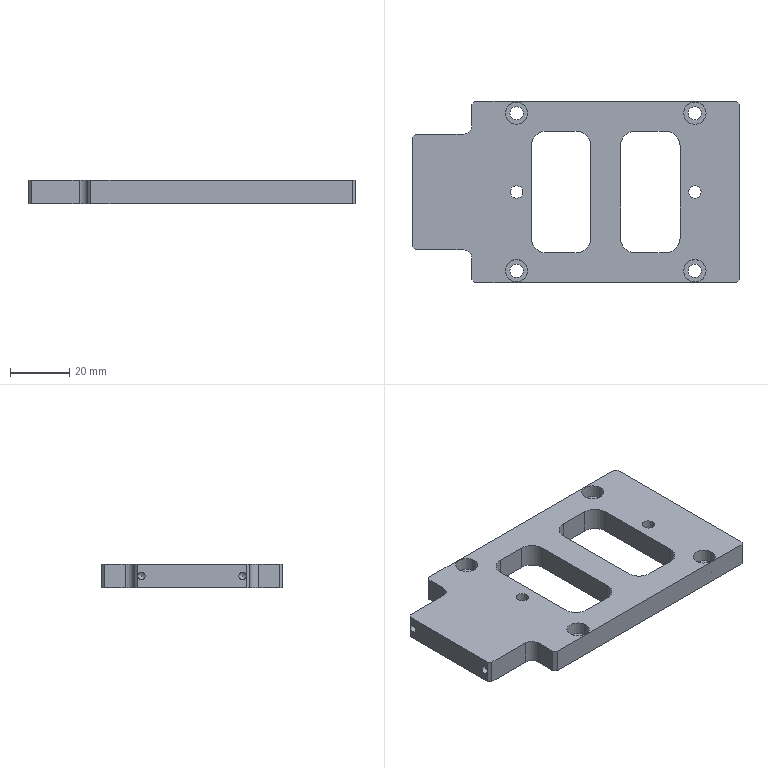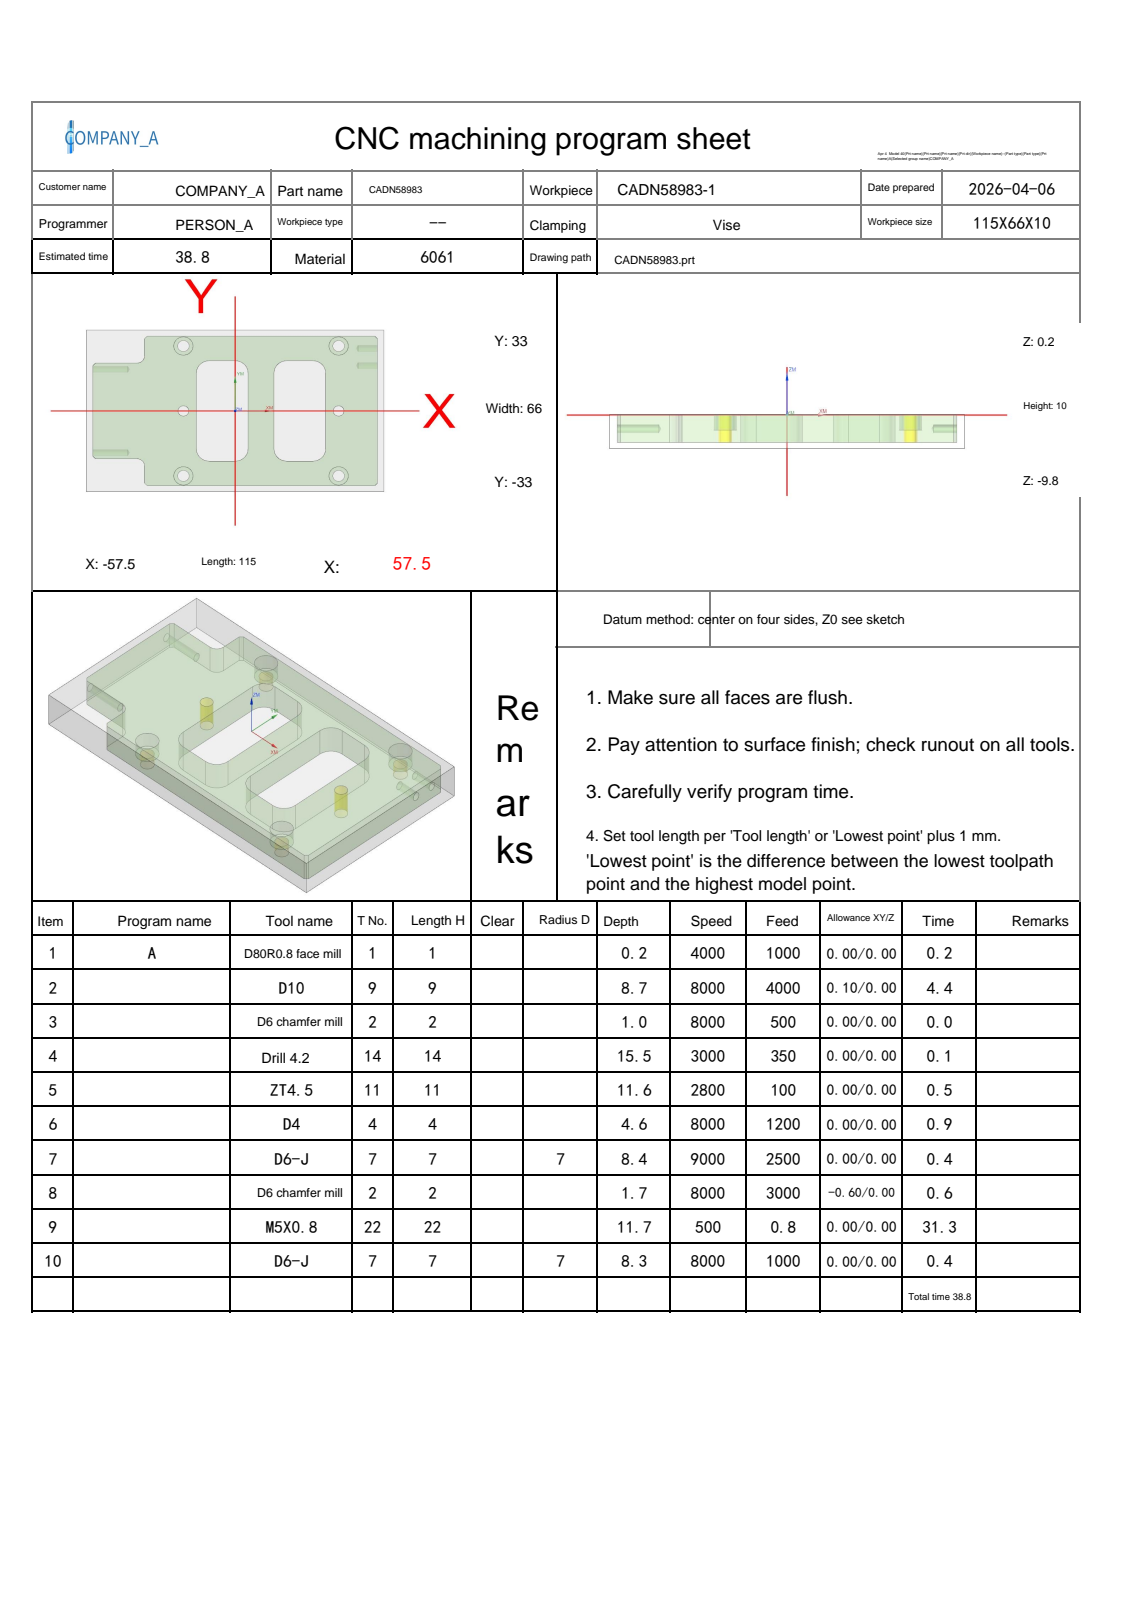NC program | NX | posted by the shop | part box 110 x 61 x 8 mm
Lines 35 to 2240 of 4510, first 1627 of 2206 lines:
N2 T09 M06
(D10  D=10. R=0. H=09 ce=0.10 di=0.10)
G00 G90 G54 X-39.25 Y-45. M03 S8000
G43 H09 Z10.2
M08
Z.724
G01 Z-.476 F4000.
Y-40.5
G03 X-46.25 Y-33.5 I-7. J0.0
G01 X-57.5
G02 X-58. Y-33. I0.0 J.5
G01 Y-24.623
G02 X-58.573 Y-24.119 I4. J5.123
X-59.617 Y-23.075 I9.382 J10.426
X-60.964 Y-21.085 I4.617 J4.575
X-61.5 Y-18.531 I5.813 J2.553
G01 Y-18.5
Y18.5
G02 X-61.492 Y18.823 I6.5 J0.0
X-60.858 Y21.317 I6.306 J-.276
X-59.618 Y23.075 I5.858 J-2.817
X-58.532 Y24.159 I10.618 J-9.54
X-58. Y24.623 I4.532 J-4.659
G01 Y33.
G02 X-57.5 Y33.5 I.5 J0.0
G01 X-41.699
G02 X-40.699 Y32.5 I0.0 J-1.
G01 X-40.713 Y32.333
X-41.614 Y27.005
X-41.627 Y26.838
G03 X-41.521 Y26.39 I1. J0.0
G01 X-41.5 Y26.301
Y26.199
G02 X-41.699 Y26. I-.2 J.001
G01 X-50.801
G02 X-51. Y26.199 I.001 J.2
G01 Y26.301
G02 X-50.801 Y26.5 I.2 J-.001
G01 X-44.983
G03 X-44.012 Y27.262 I0.0 J1.
G01 X-42.67 Y32.738
G02 X-41.699 Y33.5 I.971 J-.238
G01 X-40.123
G02 X-39.616 Y34.077 I5.123 J-4.
X-38.581 Y35.111 I11.116 J-10.081
X-36.645 Y36.438 I4.581 J-4.611
X-34.026 Y37. I2.619 J-5.815
G01 X54.
G02 X58.631 Y35.062 I0.0 J-6.5
G01 X59.596 Y34.096
G02 X61.482 Y29.977 I-4.596 J-4.596
X61.5 Y29.496 I-6.49 J-.482
G01 Y29.432
Y-29.5
G02 X59.596 Y-34.096 I-6.5 J0.0
G01 X58.596 Y-35.096
G02 X54. Y-37. I-4.596 J4.596
G01 X-34.
G02 X-38.596 Y-35.096 I0.0 J6.5
G01 X-39.596 Y-34.096
G02 X-40.123 Y-33.5 I4.596 J4.596
G01 X-51.25
G02 X-52.25 Y-32.5 I0.0 J1.
G01 X-52.23 Y-32.302
X-51.011 Y-26.253
X-50.999 Y-26.176
G02 X-50.801 Y-26. I.199 J-.024
G01 X-41.699
G02 X-41.524 Y-26.105 I-.001 J-.2
G03 X-41.134 Y-26.475 I.761 J.412
G01 X-40.7 Y-26.681
X-40.52 Y-26.721
G03 X-40.1 Y-26.301 I0.0 J.42
G01 Y-24.6
X-54.
G02 X-57.611 Y-23.101 I0.0 J5.1
X-58.606 Y-22.106 I8.417 J9.412
X-59.681 Y-20.525 I3.606 J3.606
X-60.1 Y-18.531 I4.53 J1.994
G01 Y-18.5
Y18.5
G02 X-60.093 Y18.758 I5.1 J0.0
X-59.598 Y20.707 I4.907 J-.21
X-58.6 Y22.113 I4.598 J-2.207
X-57.575 Y23.137 I9.6 J-8.578
X-55.309 Y24.429 I3.575 J-3.637
X-54.413 Y24.583 I1.296 J-4.856
X-54. Y24.6 I.413 J-5.083
G01 X-40.1
Y29.501
G02 X-40.092 Y29.79 I5.048 J0.0
X-38.6 Y33.112 I5.092 J-.29
X-37.606 Y34.106 I10.106 J-9.112
X-36.073 Y35.16 I3.606 J-3.606
X-34.026 Y35.6 I2.046 J-4.537
G01 X54.
G02 X57.641 Y34.072 I0.0 J-5.1
G01 X58.606 Y33.106
G02 X60.086 Y29.873 I-3.606 J-3.606
X60.1 Y29.496 I-5.094 J-.378
G01 Y29.439
Y-29.5
G02 X58.606 Y-33.106 I-5.1 J0.0
G01 X57.606 Y-34.106
G02 X54. Y-35.6 I-3.606 J3.606
G01 X-34.
G02 X-37.606 Y-34.106 I0.0 J5.1
G01 X-38.606 Y-33.106
G02 X-40.1 Y-29.5 I3.606 J3.606
G01 Y-26.301
G03 X-40.52 Y-25.881 I-.42 J0.0
G01 X-40.7 Y-25.922
X-41.346 Y-26.228
G03 X-41.525 Y-26.396 I.172 J-.361
G02 X-41.699 Y-26.5 I-.175 J.096
G01 X-46.25
X-50.812
G02 X-51. Y-26.301 I.012 J.2
G01 Y-26.199
X-50.976 Y-26.106
Z.724
G00 Z3.
G01 X-39.25 Y-45. F6000.
G00 Z.247
G01 Z-.953 F4000.
Y-40.5
G03 X-46.25 Y-33.5 I-7. J0.0
G01 X-57.5
G02 X-58. Y-33. I0.0 J.5
G01 Y-24.623
G02 X-58.573 Y-24.119 I4. J5.123
X-59.617 Y-23.075 I9.382 J10.426
X-60.964 Y-21.085 I4.617 J4.575
X-61.5 Y-18.531 I5.813 J2.553
G01 Y-18.5
Y18.5
G02 X-61.492 Y18.823 I6.5 J0.0
X-60.858 Y21.317 I6.306 J-.276
X-59.618 Y23.075 I5.858 J-2.817
X-58.532 Y24.159 I10.618 J-9.54
X-58. Y24.623 I4.532 J-4.659
G01 Y33.
G02 X-57.5 Y33.5 I.5 J0.0
G01 X-41.699
G02 X-40.699 Y32.5 I0.0 J-1.
G01 X-40.713 Y32.333
X-41.613 Y27.004
X-41.627 Y26.838
G03 X-41.521 Y26.39 I1. J0.0
G01 X-41.5 Y26.301
Y26.199
G02 X-41.699 Y26. I-.2 J.001
G01 X-50.801
G02 X-51. Y26.199 I.001 J.2
G01 Y26.301
G02 X-50.801 Y26.5 I.2 J-.001
G01 X-44.983
G03 X-44.012 Y27.262 I0.0 J1.
G01 X-42.67 Y32.738
G02 X-41.699 Y33.5 I.971 J-.238
G01 X-40.123
G02 X-39.616 Y34.077 I5.123 J-4.
X-38.581 Y35.111 I11.116 J-10.081
X-36.645 Y36.438 I4.581 J-4.611
X-34.026 Y37. I2.619 J-5.815
G01 X-34.
X54.
G02 X58.596 Y35.096 I0.0 J-6.5
G01 X59.596 Y34.096
G02 X61.482 Y29.977 I-4.596 J-4.596
X61.5 Y29.496 I-6.49 J-.482
G01 Y29.432
Y-29.5
G02 X59.596 Y-34.096 I-6.5 J0.0
G01 X58.596 Y-35.096
G02 X54. Y-37. I-4.596 J4.596
G01 X-34.
G02 X-38.596 Y-35.096 I0.0 J6.5
G01 X-39.596 Y-34.096
G02 X-40.123 Y-33.5 I4.596 J4.596
G01 X-51.25
G02 X-52.25 Y-32.5 I0.0 J1.
G01 X-52.23 Y-32.302
X-51.011 Y-26.253
X-50.999 Y-26.176
G02 X-50.801 Y-26. I.199 J-.024
G01 X-41.699
G02 X-41.524 Y-26.105 I-.001 J-.2
G03 X-41.134 Y-26.475 I.761 J.412
G01 X-40.7 Y-26.681
X-40.52 Y-26.721
G03 X-40.1 Y-26.301 I0.0 J.42
G01 Y-24.6
X-54.
G02 X-57.611 Y-23.101 I0.0 J5.1
X-58.606 Y-22.106 I8.417 J9.412
X-59.681 Y-20.525 I3.606 J3.606
X-60.1 Y-18.531 I4.53 J1.994
G01 Y-18.5
Y18.5
G02 X-60.093 Y18.758 I5.1 J0.0
X-59.598 Y20.707 I4.907 J-.21
X-58.6 Y22.113 I4.598 J-2.207
X-57.575 Y23.137 I9.6 J-8.578
X-55.308 Y24.429 I3.575 J-3.637
X-54.413 Y24.583 I1.296 J-4.856
X-54. Y24.6 I.413 J-5.083
G01 X-40.1
Y29.501
G02 X-40.092 Y29.79 I5.048 J0.0
X-38.6 Y33.112 I5.092 J-.29
X-37.606 Y34.106 I10.106 J-9.112
X-36.073 Y35.16 I3.606 J-3.606
X-34.026 Y35.6 I2.047 J-4.537
G01 X-34.
X54.
G02 X57.606 Y34.106 I0.0 J-5.1
G01 X58.606 Y33.106
G02 X60.086 Y29.873 I-3.606 J-3.606
X60.1 Y29.496 I-5.094 J-.378
G01 Y29.439
Y-29.5
G02 X58.606 Y-33.106 I-5.1 J0.0
G01 X57.606 Y-34.106
G02 X54. Y-35.6 I-3.606 J3.606
G01 X-34.
G02 X-37.606 Y-34.106 I0.0 J5.1
G01 X-38.606 Y-33.106
G02 X-40.1 Y-29.5 I3.606 J3.606
G01 Y-26.301
G03 X-40.52 Y-25.881 I-.42 J0.0
G01 X-40.7 Y-25.922
X-41.346 Y-26.228
G03 X-41.525 Y-26.396 I.172 J-.361
G02 X-41.699 Y-26.5 I-.175 J.096
G01 X-46.25
X-50.812
G02 X-51. Y-26.301 I.012 J.2
G01 Y-26.199
X-50.976 Y-26.106
Z.247
G00 Z2.524
G01 X-39.25 Y-45. F6000.
G00 Z-.229
G01 Z-1.429 F4000.
Y-40.5
G03 X-46.25 Y-33.5 I-7. J0.0
G01 X-57.5
G02 X-58. Y-33. I0.0 J.5
G01 Y-24.623
G02 X-58.573 Y-24.119 I4. J5.123
X-59.617 Y-23.075 I9.382 J10.426
X-60.964 Y-21.085 I4.617 J4.575
X-61.5 Y-18.531 I5.813 J2.553
G01 Y-18.5
Y18.5
G02 X-61.492 Y18.823 I6.5 J0.0
X-60.858 Y21.317 I6.306 J-.276
X-59.618 Y23.075 I5.858 J-2.817
X-58.532 Y24.159 I10.618 J-9.54
X-58. Y24.623 I4.532 J-4.659
G01 Y33.
G02 X-57.5 Y33.5 I.5 J0.0
G01 X-41.699
G02 X-40.699 Y32.5 I0.0 J-1.
G01 X-40.713 Y32.333
X-41.613 Y27.004
X-41.627 Y26.838
G03 X-41.521 Y26.39 I1. J0.0
G01 X-41.5 Y26.301
Y26.199
G02 X-41.699 Y26. I-.2 J.001
G01 X-50.801
G02 X-51. Y26.199 I.001 J.2
G01 Y26.301
G02 X-50.801 Y26.5 I.2 J-.001
G01 X-44.983
G03 X-44.012 Y27.262 I0.0 J1.
G01 X-42.67 Y32.738
G02 X-41.699 Y33.5 I.971 J-.238
G01 X-40.123
G02 X-39.616 Y34.077 I5.123 J-4.
X-38.581 Y35.111 I11.116 J-10.081
X-36.645 Y36.438 I4.581 J-4.611
X-34.026 Y37. I2.619 J-5.815
G01 X-34.
X54.
G02 X58.596 Y35.096 I0.0 J-6.5
G01 X59.596 Y34.096
G02 X61.482 Y29.977 I-4.596 J-4.596
X61.5 Y29.496 I-6.49 J-.481
G01 Y29.432
Y-29.5
G02 X59.596 Y-34.096 I-6.5 J0.0
G01 X58.596 Y-35.096
G02 X54. Y-37. I-4.596 J4.596
G01 X-34.
G02 X-38.596 Y-35.096 I0.0 J6.5
G01 X-39.596 Y-34.096
G02 X-40.123 Y-33.5 I4.596 J4.596
G01 X-51.25
G02 X-52.25 Y-32.5 I0.0 J1.
G01 X-52.23 Y-32.302
X-51.011 Y-26.253
X-50.999 Y-26.176
G02 X-50.801 Y-26. I.199 J-.024
G01 X-41.699
G02 X-41.524 Y-26.105 I-.001 J-.2
G03 X-41.134 Y-26.475 I.761 J.412
G01 X-40.7 Y-26.681
X-40.52 Y-26.721
G03 X-40.1 Y-26.301 I0.0 J.42
G01 Y-24.6
X-54.
G02 X-57.611 Y-23.101 I0.0 J5.1
X-58.606 Y-22.106 I8.417 J9.412
X-59.681 Y-20.525 I3.606 J3.606
X-60.1 Y-18.531 I4.53 J1.994
G01 Y-18.5
Y18.5
G02 X-60.093 Y18.758 I5.1 J0.0
X-59.598 Y20.707 I4.907 J-.21
X-58.6 Y22.113 I4.598 J-2.207
X-57.575 Y23.137 I9.6 J-8.578
X-55.308 Y24.429 I3.575 J-3.637
X-54.413 Y24.583 I1.296 J-4.856
X-54. Y24.6 I.413 J-5.083
G01 X-40.1
Y29.501
G02 X-40.092 Y29.79 I5.048 J0.0
X-38.6 Y33.112 I5.092 J-.29
X-37.606 Y34.106 I10.106 J-9.112
X-36.073 Y35.16 I3.606 J-3.606
X-34.026 Y35.6 I2.046 J-4.537
G01 X-34.
X54.
G02 X57.606 Y34.106 I0.0 J-5.1
G01 X58.606 Y33.106
G02 X60.086 Y29.873 I-3.606 J-3.606
X60.1 Y29.496 I-5.094 J-.378
G01 Y29.439
Y-29.5
G02 X58.606 Y-33.106 I-5.1 J0.0
G01 X57.606 Y-34.106
G02 X54. Y-35.6 I-3.606 J3.606
G01 X-34.
G02 X-37.606 Y-34.106 I0.0 J5.1
G01 X-38.606 Y-33.106
G02 X-40.1 Y-29.5 I3.606 J3.606
G01 Y-26.301
G03 X-40.52 Y-25.881 I-.42 J0.0
G01 X-40.7 Y-25.922
X-41.346 Y-26.228
G03 X-41.525 Y-26.396 I.172 J-.361
G02 X-41.699 Y-26.5 I-.175 J.096
G01 X-46.25
X-50.812
G02 X-51. Y-26.301 I.012 J.2
G01 Y-26.199
X-50.976 Y-26.106
Z-.229
G00 Z2.047
G01 X-39.25 Y-45. F6000.
G00 Z-.706
G01 Z-1.906 F4000.
Y-40.5
G03 X-46.25 Y-33.5 I-7. J0.0
G01 X-57.5
G02 X-58. Y-33. I0.0 J.5
G01 Y-24.623
G02 X-58.573 Y-24.119 I4. J5.123
X-59.617 Y-23.075 I9.382 J10.426
X-60.964 Y-21.085 I4.617 J4.575
X-61.5 Y-18.531 I5.813 J2.553
G01 Y-18.5
Y18.5
G02 X-61.492 Y18.823 I6.5 J0.0
X-60.858 Y21.317 I6.306 J-.276
X-59.618 Y23.075 I5.858 J-2.817
X-58.532 Y24.159 I10.618 J-9.54
X-58. Y24.623 I4.532 J-4.659
G01 Y33.
G02 X-57.5 Y33.5 I.5 J0.0
G01 X-41.699
G02 X-40.699 Y32.5 I0.0 J-1.
G01 X-40.713 Y32.333
X-41.613 Y27.004
X-41.627 Y26.838
G03 X-41.521 Y26.39 I1. J0.0
G01 X-41.5 Y26.301
Y26.199
G02 X-41.699 Y26. I-.2 J.001
G01 X-50.801
G02 X-51. Y26.199 I.001 J.2
G01 Y26.301
G02 X-50.801 Y26.5 I.2 J-.001
G01 X-44.983
G03 X-44.012 Y27.262 I0.0 J1.
G01 X-42.67 Y32.738
G02 X-41.699 Y33.5 I.971 J-.238
G01 X-40.123
G02 X-39.616 Y34.077 I5.123 J-4.
X-38.581 Y35.111 I11.116 J-10.081
X-36.645 Y36.438 I4.581 J-4.611
X-34.026 Y37. I2.619 J-5.815
G01 X-34.
X54.
G02 X58.596 Y35.096 I0.0 J-6.5
G01 X59.596 Y34.096
G02 X61.482 Y29.977 I-4.596 J-4.596
X61.5 Y29.496 I-6.49 J-.481
G01 Y29.432
Y-29.5
G02 X59.596 Y-34.096 I-6.5 J0.0
G01 X58.596 Y-35.096
G02 X54. Y-37. I-4.596 J4.596
G01 X-34.
G02 X-38.596 Y-35.096 I0.0 J6.5
G01 X-39.596 Y-34.096
G02 X-40.123 Y-33.5 I4.596 J4.596
G01 X-51.25
G02 X-52.25 Y-32.5 I0.0 J1.
G01 X-52.23 Y-32.302
X-51.011 Y-26.253
X-50.999 Y-26.176
G02 X-50.801 Y-26. I.199 J-.024
G01 X-41.699
G02 X-41.524 Y-26.105 I-.001 J-.2
G03 X-41.134 Y-26.475 I.761 J.412
G01 X-40.7 Y-26.681
X-40.52 Y-26.721
G03 X-40.1 Y-26.301 I0.0 J.42
G01 Y-24.6
X-54.
G02 X-57.611 Y-23.101 I0.0 J5.1
X-58.606 Y-22.106 I8.417 J9.412
X-59.681 Y-20.525 I3.606 J3.606
X-60.1 Y-18.531 I4.53 J1.994
G01 Y-18.5
Y18.5
G02 X-60.093 Y18.758 I5.1 J0.0
X-59.598 Y20.707 I4.907 J-.21
X-58.6 Y22.113 I4.598 J-2.207
X-57.575 Y23.137 I9.6 J-8.578
X-55.308 Y24.429 I3.575 J-3.637
X-54.413 Y24.583 I1.296 J-4.856
X-54. Y24.6 I.413 J-5.083
G01 X-40.1
Y29.501
G02 X-40.092 Y29.789 I5.048 J0.0
X-38.6 Y33.112 I5.092 J-.289
X-37.606 Y34.106 I10.106 J-9.112
X-36.072 Y35.16 I3.606 J-3.606
X-34.026 Y35.6 I2.046 J-4.537
G01 X-34.
X54.
G02 X57.606 Y34.106 I0.0 J-5.1
G01 X58.606 Y33.106
G02 X60.086 Y29.873 I-3.606 J-3.606
X60.1 Y29.496 I-5.094 J-.378
G01 Y29.439
Y-29.5
G02 X58.606 Y-33.106 I-5.1 J0.0
G01 X57.606 Y-34.106
G02 X54. Y-35.6 I-3.606 J3.606
G01 X-34.
G02 X-37.606 Y-34.106 I0.0 J5.1
G01 X-38.606 Y-33.106
G02 X-40.1 Y-29.5 I3.606 J3.606
G01 Y-26.301
G03 X-40.52 Y-25.881 I-.42 J0.0
G01 X-40.7 Y-25.922
X-41.346 Y-26.229
G03 X-41.525 Y-26.397 I.172 J-.361
G02 X-41.699 Y-26.5 I-.175 J.097
G01 X-46.25
X-50.812
G02 X-51. Y-26.301 I.012 J.2
G01 Y-26.199
X-50.976 Y-26.106
Z-.706
G00 Z1.571
G01 X-39.25 Y-45. F6000.
G00 Z-1.182
G01 Z-2.382 F4000.
Y-40.5
G03 X-46.25 Y-33.5 I-7. J0.0
G01 X-57.5
G02 X-58. Y-33. I0.0 J.5
G01 Y-24.623
G02 X-58.573 Y-24.119 I4. J5.123
X-59.617 Y-23.075 I9.382 J10.426
X-60.964 Y-21.085 I4.617 J4.575
X-61.5 Y-18.531 I5.813 J2.553
G01 Y-18.5
Y18.5
G02 X-61.492 Y18.823 I6.5 J0.0
X-60.858 Y21.317 I6.306 J-.276
X-59.618 Y23.075 I5.858 J-2.817
X-58.532 Y24.159 I10.618 J-9.54
X-58. Y24.623 I4.532 J-4.659
G01 Y33.
G02 X-57.5 Y33.5 I.5 J0.0
G01 X-41.698
G02 X-40.698 Y32.5 I0.0 J-1.
G01 X-40.712 Y32.333
X-41.613 Y27.004
X-41.627 Y26.838
G03 X-41.521 Y26.39 I1. J0.0
G01 X-41.5 Y26.302
Y26.198
G02 X-41.698 Y26. I-.2 J.002
G01 X-50.802
G02 X-51. Y26.198 I.002 J.2
G01 Y26.302
G02 X-50.802 Y26.5 I.2 J-.002
G01 X-44.983
G03 X-44.012 Y27.262 I0.0 J1.
G01 X-42.67 Y32.738
G02 X-41.698 Y33.5 I.971 J-.238
G01 X-40.123
G02 X-39.616 Y34.077 I5.123 J-4.
X-38.581 Y35.111 I11.116 J-10.081
X-36.645 Y36.438 I4.581 J-4.611
X-34.026 Y37. I2.619 J-5.815
G01 X-34.
X54.
G02 X58.596 Y35.096 I0.0 J-6.5
G01 X59.596 Y34.096
G02 X61.482 Y29.977 I-4.596 J-4.596
X61.5 Y29.496 I-6.49 J-.481
G01 Y29.432
Y-29.5
G02 X59.596 Y-34.096 I-6.5 J0.0
G01 X58.596 Y-35.096
G02 X54. Y-37. I-4.596 J4.596
G01 X-34.
G02 X-38.596 Y-35.096 I0.0 J6.5
G01 X-39.596 Y-34.096
G02 X-40.123 Y-33.5 I4.596 J4.596
G01 X-51.25
G02 X-52.25 Y-32.5 I0.0 J1.
G01 X-52.23 Y-32.302
X-51.011 Y-26.253
X-50.999 Y-26.176
G02 X-50.802 Y-26. I.199 J-.024
G01 X-41.698
G02 X-41.524 Y-26.105 I-.002 J-.2
G03 X-41.134 Y-26.475 I.761 J.412
G01 X-40.7 Y-26.681
X-40.52 Y-26.722
G03 X-40.1 Y-26.302 I0.0 J.42
G01 Y-24.6
X-54.
G02 X-57.611 Y-23.101 I0.0 J5.1
X-58.606 Y-22.106 I8.417 J9.412
X-59.681 Y-20.525 I3.606 J3.606
X-60.1 Y-18.531 I4.53 J1.994
G01 Y-18.5
Y18.5
G02 X-60.093 Y18.758 I5.1 J0.0
X-59.598 Y20.707 I4.907 J-.21
X-58.6 Y22.113 I4.598 J-2.207
X-57.575 Y23.137 I9.6 J-8.578
X-55.308 Y24.429 I3.575 J-3.637
X-54.413 Y24.583 I1.296 J-4.856
X-54. Y24.6 I.413 J-5.083
G01 X-40.1
Y29.501
G02 X-40.092 Y29.789 I5.048 J0.0
X-38.6 Y33.112 I5.092 J-.289
X-37.606 Y34.106 I10.106 J-9.112
X-36.072 Y35.16 I3.606 J-3.606
X-34.026 Y35.6 I2.046 J-4.537
G01 X-34.
X54.
G02 X57.606 Y34.106 I0.0 J-5.1
G01 X58.606 Y33.106
G02 X60.086 Y29.873 I-3.606 J-3.606
X60.1 Y29.496 I-5.094 J-.378
G01 Y29.439
Y-29.5
G02 X58.606 Y-33.106 I-5.1 J0.0
G01 X57.606 Y-34.106
G02 X54. Y-35.6 I-3.606 J3.606
G01 X-34.
G02 X-37.606 Y-34.106 I0.0 J5.1
G01 X-38.606 Y-33.106
G02 X-40.1 Y-29.5 I3.606 J3.606
G01 Y-26.302
G03 X-40.52 Y-25.882 I-.42 J0.0
G01 X-40.7 Y-25.922
X-41.346 Y-26.229
G03 X-41.525 Y-26.397 I.172 J-.361
G02 X-41.698 Y-26.5 I-.175 J.097
G01 X-46.25
X-50.812
G02 X-51. Y-26.302 I.012 J.2
G01 Y-26.198
X-50.976 Y-26.106
Z-1.182
G00 Z1.094
G01 X-39.25 Y-45. F6000.
G00 Z-1.659
G01 Z-2.859 F4000.
Y-40.5
G03 X-46.25 Y-33.5 I-7. J0.0
G01 X-57.5
G02 X-58. Y-33. I0.0 J.5
G01 Y-24.623
G02 X-58.573 Y-24.119 I4. J5.123
X-59.617 Y-23.075 I9.382 J10.426
X-60.964 Y-21.085 I4.617 J4.575
X-61.5 Y-18.531 I5.813 J2.553
G01 Y-18.5
Y18.5
G02 X-61.492 Y18.823 I6.5 J0.0
X-60.858 Y21.317 I6.306 J-.276
X-59.618 Y23.075 I5.858 J-2.817
X-58.532 Y24.159 I10.618 J-9.54
X-58. Y24.623 I4.532 J-4.659
G01 Y33.
G02 X-57.5 Y33.5 I.5 J0.0
G01 X-41.698
G02 X-40.698 Y32.5 I0.0 J-1.
G01 X-40.712 Y32.333
X-41.613 Y27.004
X-41.627 Y26.838
G03 X-41.521 Y26.39 I1. J0.0
G01 X-41.5 Y26.302
Y26.198
G02 X-41.698 Y26. I-.2 J.002
G01 X-50.802
G02 X-51. Y26.198 I.002 J.2
G01 Y26.302
G02 X-50.802 Y26.5 I.2 J-.002
G01 X-44.983
G03 X-44.012 Y27.262 I0.0 J1.
G01 X-42.67 Y32.738
G02 X-41.698 Y33.5 I.971 J-.238
G01 X-40.123
G02 X-39.616 Y34.077 I5.123 J-4.
X-38.581 Y35.111 I11.116 J-10.081
X-36.645 Y36.438 I4.581 J-4.611
X-34.026 Y37. I2.619 J-5.815
G01 X-34.
X54.
G02 X58.596 Y35.096 I0.0 J-6.5
G01 X59.596 Y34.096
G02 X61.483 Y29.977 I-4.596 J-4.596
X61.5 Y29.496 I-6.49 J-.481
G01 Y29.432
Y-29.5
G02 X59.596 Y-34.096 I-6.5 J0.0
G01 X58.596 Y-35.096
G02 X54. Y-37. I-4.596 J4.596
G01 X-34.
G02 X-38.596 Y-35.096 I0.0 J6.5
G01 X-39.596 Y-34.096
G02 X-40.123 Y-33.5 I4.596 J4.596
G01 X-51.25
G02 X-52.25 Y-32.5 I0.0 J1.
G01 X-52.23 Y-32.302
X-51.011 Y-26.252
X-50.999 Y-26.176
G02 X-50.802 Y-26. I.199 J-.024
G01 X-41.698
G02 X-41.524 Y-26.105 I-.002 J-.2
G03 X-41.134 Y-26.475 I.761 J.412
G01 X-40.7 Y-26.681
X-40.52 Y-26.722
G03 X-40.1 Y-26.302 I0.0 J.42
G01 Y-24.6
X-54.
G02 X-57.611 Y-23.101 I0.0 J5.1
X-58.606 Y-22.106 I8.417 J9.412
X-59.681 Y-20.525 I3.606 J3.606
X-60.1 Y-18.531 I4.53 J1.994
G01 Y-18.5
Y18.5
G02 X-60.093 Y18.758 I5.1 J0.0
X-59.598 Y20.707 I4.907 J-.21
X-58.6 Y22.113 I4.598 J-2.207
X-57.575 Y23.137 I9.6 J-8.578
X-55.308 Y24.429 I3.575 J-3.637
X-54.413 Y24.583 I1.296 J-4.856
X-54. Y24.6 I.413 J-5.083
G01 X-40.1
Y29.502
X-40.092 Y29.789
G02 X-38.6 Y33.112 I5.092 J-.289
X-37.606 Y34.106 I10.106 J-9.112
X-36.072 Y35.16 I3.606 J-3.606
X-34.026 Y35.6 I2.046 J-4.537
G01 X-34.
X54.
G02 X57.606 Y34.106 I0.0 J-5.1
G01 X58.606 Y33.106
G02 X60.086 Y29.873 I-3.606 J-3.606
X60.1 Y29.496 I-5.094 J-.378
G01 Y29.439
Y-29.5
G02 X58.606 Y-33.106 I-5.1 J0.0
G01 X57.606 Y-34.106
G02 X54. Y-35.6 I-3.606 J3.606
G01 X-34.
G02 X-37.606 Y-34.106 I0.0 J5.1
G01 X-38.606 Y-33.106
G02 X-40.1 Y-29.5 I3.606 J3.606
G01 Y-26.302
G03 X-40.52 Y-25.882 I-.42 J0.0
G01 X-40.7 Y-25.922
X-41.346 Y-26.229
G03 X-41.525 Y-26.397 I.172 J-.361
G02 X-41.698 Y-26.5 I-.175 J.097
G01 X-46.25
X-50.812
G02 X-51. Y-26.302 I.012 J.2
G01 Y-26.198
X-50.976 Y-26.106
Z-1.659
G00 Z.618
G01 X-39.25 Y-45. F6000.
G00 Z-2.135
G01 Z-3.335 F4000.
Y-40.5
G03 X-46.25 Y-33.5 I-7. J0.0
G01 X-57.5
G02 X-58. Y-33. I0.0 J.5
G01 Y-24.623
G02 X-58.573 Y-24.119 I4. J5.123
X-59.617 Y-23.075 I9.382 J10.426
X-60.964 Y-21.085 I4.617 J4.575
X-61.5 Y-18.531 I5.813 J2.553
G01 Y-18.5
Y18.5
G02 X-61.492 Y18.823 I6.5 J0.0
X-60.858 Y21.317 I6.306 J-.276
X-59.618 Y23.075 I5.858 J-2.817
X-58.532 Y24.159 I10.618 J-9.54
X-58. Y24.623 I4.532 J-4.659
G01 Y33.
G02 X-57.5 Y33.5 I.5 J0.0
G01 X-41.698
G02 X-40.698 Y32.5 I0.0 J-1.
G01 X-40.712 Y32.333
X-41.613 Y27.004
X-41.627 Y26.837
G03 X-41.521 Y26.39 I1. J0.0
G01 X-41.5 Y26.302
Y26.198
G02 X-41.698 Y26. I-.2 J.002
G01 X-50.802
G02 X-51. Y26.198 I.002 J.2
G01 Y26.302
G02 X-50.802 Y26.5 I.2 J-.002
G01 X-44.983
G03 X-44.012 Y27.262 I0.0 J1.
G01 X-42.67 Y32.738
G02 X-41.698 Y33.5 I.971 J-.238
G01 X-40.123
G02 X-39.616 Y34.077 I5.123 J-4.
X-38.581 Y35.111 I11.116 J-10.081
X-36.645 Y36.438 I4.581 J-4.611
X-34.026 Y37. I2.619 J-5.815
G01 X-34.
X54.
G02 X58.596 Y35.096 I0.0 J-6.5
G01 X59.596 Y34.096
G02 X61.483 Y29.977 I-4.596 J-4.596
X61.5 Y29.496 I-6.49 J-.481
G01 Y29.432
Y-29.5
G02 X59.596 Y-34.096 I-6.5 J0.0
G01 X58.596 Y-35.096
G02 X54. Y-37. I-4.596 J4.596
G01 X-34.
G02 X-38.596 Y-35.096 I0.0 J6.5
G01 X-39.596 Y-34.096
G02 X-40.123 Y-33.5 I4.596 J4.596
G01 X-51.25
G02 X-52.25 Y-32.5 I0.0 J1.
G01 X-52.23 Y-32.302
X-51.011 Y-26.252
X-50.999 Y-26.176
G02 X-50.802 Y-26. I.199 J-.024
G01 X-41.698
G02 X-41.524 Y-26.105 I-.002 J-.2
G03 X-41.134 Y-26.475 I.761 J.412
G01 X-40.7 Y-26.681
X-40.52 Y-26.722
G03 X-40.1 Y-26.302 I0.0 J.42
G01 Y-24.6
X-54.
G02 X-57.611 Y-23.101 I0.0 J5.1
X-58.606 Y-22.106 I8.417 J9.412
X-59.681 Y-20.525 I3.606 J3.606
X-60.1 Y-18.531 I4.53 J1.994
G01 Y-18.5
Y18.5
G02 X-60.093 Y18.758 I5.1 J0.0
X-59.598 Y20.707 I4.907 J-.21
X-58.6 Y22.113 I4.598 J-2.207
X-57.575 Y23.137 I9.6 J-8.578
X-55.308 Y24.429 I3.575 J-3.637
X-54.413 Y24.583 I1.296 J-4.856
X-54. Y24.6 I.413 J-5.083
G01 X-40.1
Y29.5
G02 X-38.6 Y33.112 I5.1 J0.0
X-37.606 Y34.106 I10.106 J-9.112
X-36.072 Y35.16 I3.606 J-3.606
X-34.026 Y35.6 I2.046 J-4.537
G01 X-34.
X54.
G02 X57.606 Y34.106 I0.0 J-5.1
G01 X58.606 Y33.106
G02 X60.086 Y29.873 I-3.606 J-3.606
X60.1 Y29.496 I-5.094 J-.378
G01 Y29.439
Y-29.5
G02 X58.606 Y-33.106 I-5.1 J0.0
G01 X57.606 Y-34.106
G02 X54. Y-35.6 I-3.606 J3.606
G01 X-34.
G02 X-37.606 Y-34.106 I0.0 J5.1
G01 X-38.606 Y-33.106
G02 X-40.1 Y-29.5 I3.606 J3.606
G01 Y-26.302
G03 X-40.52 Y-25.882 I-.42 J0.0
G01 X-40.7 Y-25.922
X-41.346 Y-26.229
G03 X-41.525 Y-26.397 I.172 J-.361
G02 X-41.698 Y-26.5 I-.175 J.097
G01 X-46.25
X-50.812
G02 X-51. Y-26.302 I.012 J.2
G01 Y-26.198
X-50.976 Y-26.106
Z-2.135
G00 Z.141
G01 X-39.25 Y-45. F6000.
G00 Z-2.612
G01 Z-3.812 F4000.
Y-40.5
G03 X-46.25 Y-33.5 I-7. J0.0
G01 X-57.5
G02 X-58. Y-33. I0.0 J.5
G01 Y-24.623
G02 X-58.573 Y-24.119 I4. J5.123
X-59.617 Y-23.075 I9.382 J10.426
X-60.964 Y-21.085 I4.617 J4.575
X-61.5 Y-18.531 I5.813 J2.553
G01 Y-18.5
Y18.5
G02 X-61.492 Y18.823 I6.5 J0.0
X-60.858 Y21.317 I6.306 J-.276
X-59.618 Y23.075 I5.858 J-2.817
X-58.532 Y24.159 I10.618 J-9.54
X-58. Y24.623 I4.532 J-4.659
G01 Y33.
G02 X-57.5 Y33.5 I.5 J0.0
G01 X-41.698
G02 X-40.698 Y32.5 I0.0 J-1.
G01 X-40.712 Y32.333
X-41.613 Y27.004
X-41.627 Y26.837
G03 X-41.521 Y26.39 I1. J0.0
G01 X-41.5 Y26.302
Y26.198
G02 X-41.698 Y26. I-.2 J.002
G01 X-50.802
G02 X-51. Y26.198 I.002 J.2
G01 Y26.302
G02 X-50.802 Y26.5 I.2 J-.002
G01 X-44.982
G03 X-44.012 Y27.262 I0.0 J1.
G01 X-42.67 Y32.738
G02 X-41.698 Y33.5 I.971 J-.238
G01 X-40.123
G02 X-39.616 Y34.077 I5.123 J-4.
X-38.581 Y35.111 I11.116 J-10.081
X-36.645 Y36.438 I4.581 J-4.611
X-34.026 Y37. I2.619 J-5.815
G01 X-34.
X54.
G02 X58.596 Y35.096 I0.0 J-6.5
G01 X59.596 Y34.096
G02 X61.483 Y29.976 I-4.596 J-4.596
X61.5 Y29.496 I-6.49 J-.481
G01 Y29.432
Y-29.5
G02 X59.596 Y-34.096 I-6.5 J0.0
G01 X58.596 Y-35.096
G02 X54. Y-37. I-4.596 J4.596
G01 X-34.
G02 X-38.596 Y-35.096 I0.0 J6.5
G01 X-39.596 Y-34.096
G02 X-40.123 Y-33.5 I4.596 J4.596
G01 X-51.25
G02 X-52.25 Y-32.5 I0.0 J1.
G01 X-52.23 Y-32.302
X-51.011 Y-26.252
X-50.999 Y-26.176
G02 X-50.802 Y-26. I.199 J-.024
G01 X-41.698
G02 X-41.524 Y-26.105 I-.002 J-.2
G03 X-41.134 Y-26.476 I.762 J.411
G01 X-40.7 Y-26.681
X-40.52 Y-26.722
G03 X-40.1 Y-26.302 I0.0 J.42
G01 Y-24.6
X-54.
G02 X-57.611 Y-23.101 I0.0 J5.1
X-58.606 Y-22.106 I8.417 J9.412
X-59.681 Y-20.525 I3.606 J3.606
X-60.1 Y-18.531 I4.53 J1.994
G01 Y-18.5
Y18.5
G02 X-60.093 Y18.758 I5.1 J0.0
X-59.598 Y20.707 I4.907 J-.21
X-58.6 Y22.113 I4.598 J-2.207
X-57.575 Y23.137 I9.6 J-8.578
X-55.308 Y24.429 I3.575 J-3.637
X-54.413 Y24.583 I1.296 J-4.856
X-54. Y24.6 I.413 J-5.083
G01 X-40.1
Y29.5
G02 X-38.6 Y33.112 I5.1 J0.0
X-37.606 Y34.106 I10.106 J-9.112
X-36.072 Y35.16 I3.606 J-3.606
X-34.026 Y35.6 I2.046 J-4.537
G01 X-34.
X54.
G02 X57.606 Y34.106 I0.0 J-5.1
G01 X58.606 Y33.106
G02 X60.086 Y29.873 I-3.606 J-3.606
X60.1 Y29.496 I-5.094 J-.377
G01 Y29.439
Y-29.5
G02 X58.606 Y-33.106 I-5.1 J0.0
G01 X57.606 Y-34.106
G02 X54. Y-35.6 I-3.606 J3.606
G01 X-34.
G02 X-37.606 Y-34.106 I0.0 J5.1
G01 X-38.606 Y-33.106
G02 X-40.1 Y-29.5 I3.606 J3.606
G01 Y-26.302
G03 X-40.52 Y-25.882 I-.42 J0.0
G01 X-40.7 Y-25.922
X-41.346 Y-26.229
G03 X-41.525 Y-26.397 I.172 J-.361
G02 X-41.698 Y-26.5 I-.175 J.097
G01 X-46.25
X-50.812
G02 X-51. Y-26.302 I.012 J.2
G01 Y-26.198
X-50.976 Y-26.106
Z-2.612
G00 Z-.335
G01 X-39.25 Y-45. F6000.
G00 Z-3.088
G01 Z-4.288 F4000.
Y-40.5
G03 X-46.25 Y-33.5 I-7. J0.0
G01 X-57.5
G02 X-58. Y-33. I0.0 J.5
G01 Y-24.623
G02 X-58.573 Y-24.119 I4. J5.123
X-59.617 Y-23.075 I9.382 J10.426
X-60.964 Y-21.085 I4.617 J4.575
X-61.5 Y-18.531 I5.813 J2.553
G01 Y-18.5
Y18.5
G02 X-61.492 Y18.823 I6.5 J0.0
X-60.858 Y21.317 I6.306 J-.276
X-59.618 Y23.075 I5.858 J-2.817
X-58.532 Y24.159 I10.618 J-9.54
X-58. Y24.623 I4.532 J-4.659
G01 Y33.
G02 X-57.5 Y33.5 I.5 J0.0
G01 X-41.698
G02 X-40.698 Y32.5 I0.0 J-1.
G01 X-40.712 Y32.333
X-41.613 Y27.004
X-41.627 Y26.837
G03 X-41.521 Y26.39 I1. J0.0
G01 X-41.5 Y26.302
Y26.198
G02 X-41.698 Y26. I-.2 J.002
G01 X-50.802
G02 X-51. Y26.198 I.002 J.2
G01 Y26.302
G02 X-50.802 Y26.5 I.2 J-.002
G01 X-44.982
G03 X-44.012 Y27.262 I0.0 J1.
G01 X-42.669 Y32.738
G02 X-41.698 Y33.5 I.971 J-.238
G01 X-40.123
G02 X-39.616 Y34.077 I5.123 J-4.
X-38.581 Y35.111 I11.116 J-10.081
X-36.645 Y36.438 I4.581 J-4.611
X-34.026 Y37. I2.619 J-5.815
G01 X-34.
X54.
G02 X58.596 Y35.096 I0.0 J-6.5
G01 X59.596 Y34.096
G02 X61.483 Y29.976 I-4.596 J-4.596
X61.5 Y29.496 I-6.49 J-.481
G01 Y29.432
Y-29.5
G02 X59.596 Y-34.096 I-6.5 J0.0
G01 X58.596 Y-35.096
G02 X54. Y-37. I-4.596 J4.596
G01 X-34.
G02 X-38.596 Y-35.096 I0.0 J6.5
G01 X-39.596 Y-34.096
G02 X-40.123 Y-33.5 I4.596 J4.596
G01 X-51.25
G02 X-52.25 Y-32.5 I0.0 J1.
G01 X-52.23 Y-32.302
X-51.011 Y-26.252
X-50.999 Y-26.176
G02 X-50.802 Y-26. I.199 J-.024
G01 X-41.698
G02 X-41.524 Y-26.105 I-.002 J-.2
G03 X-41.134 Y-26.476 I.762 J.411
G01 X-40.7 Y-26.681
X-40.52 Y-26.722
G03 X-40.1 Y-26.302 I0.0 J.42
G01 Y-24.6
X-54.
G02 X-57.611 Y-23.101 I0.0 J5.1
X-58.606 Y-22.106 I8.417 J9.412
X-59.681 Y-20.525 I3.606 J3.606
X-60.1 Y-18.531 I4.53 J1.994
G01 Y-18.5
Y18.5
G02 X-60.093 Y18.758 I5.1 J0.0
X-59.598 Y20.707 I4.907 J-.21
X-58.6 Y22.113 I4.598 J-2.207
X-57.575 Y23.137 I9.6 J-8.578
X-55.308 Y24.429 I3.575 J-3.637
X-54.413 Y24.583 I1.296 J-4.856
X-54. Y24.6 I.413 J-5.083
G01 X-40.1
Y29.5
G02 X-38.6 Y33.112 I5.1 J0.0
X-37.606 Y34.106 I10.106 J-9.112
X-36.072 Y35.16 I3.606 J-3.606
X-34.026 Y35.6 I2.046 J-4.537
G01 X-34.
X54.
G02 X57.606 Y34.106 I0.0 J-5.1
G01 X58.606 Y33.106
G02 X60.086 Y29.873 I-3.606 J-3.606
X60.1 Y29.496 I-5.094 J-.377
G01 Y29.439
Y-29.5
G02 X58.606 Y-33.106 I-5.1 J0.0
G01 X57.606 Y-34.106
G02 X54. Y-35.6 I-3.606 J3.606
G01 X-34.
G02 X-37.606 Y-34.106 I0.0 J5.1
G01 X-38.606 Y-33.106
G02 X-40.1 Y-29.5 I3.606 J3.606
G01 Y-26.302
G03 X-40.52 Y-25.882 I-.42 J0.0
G01 X-40.7 Y-25.922
X-41.347 Y-26.229
G03 X-41.525 Y-26.397 I.172 J-.361
G02 X-41.698 Y-26.5 I-.175 J.097
G01 X-46.25
X-50.812
G02 X-51. Y-26.302 I.012 J.2
G01 Y-26.198
X-50.976 Y-26.106
Z-3.088
G00 Z-.812
G01 X-39.25 Y-45. F6000.
G00 Z-3.565
G01 Z-4.765 F4000.
Y-40.5
G03 X-46.25 Y-33.5 I-7. J0.0
G01 X-57.5
G02 X-58. Y-33. I0.0 J.5
G01 Y-24.623
G02 X-58.573 Y-24.119 I4. J5.123
X-59.617 Y-23.075 I9.382 J10.426
X-60.964 Y-21.085 I4.617 J4.575
X-61.5 Y-18.531 I5.813 J2.553
G01 Y-18.5
Y18.5
G02 X-61.492 Y18.823 I6.5 J0.0
X-60.858 Y21.317 I6.306 J-.276
X-59.618 Y23.075 I5.858 J-2.817
X-58.532 Y24.159 I10.618 J-9.54
X-58. Y24.623 I4.532 J-4.659
G01 Y33.
G02 X-57.5 Y33.5 I.5 J0.0
G01 X-41.698
G02 X-40.698 Y32.5 I0.0 J-1.
G01 X-40.712 Y32.333
X-41.613 Y27.004
X-41.627 Y26.837
G03 X-41.521 Y26.39 I1. J0.0
G01 X-41.5 Y26.302
Y26.198
G02 X-41.698 Y26. I-.2 J.002
G01 X-50.802
G02 X-51. Y26.198 I.002 J.2
G01 Y26.302
G02 X-50.802 Y26.5 I.2 J-.002
G01 X-44.982
G03 X-44.011 Y27.262 I0.0 J1.
G01 X-42.669 Y32.738
G02 X-41.698 Y33.5 I.971 J-.238
G01 X-40.123
G02 X-39.616 Y34.077 I5.123 J-4.
X-38.581 Y35.111 I11.116 J-10.081
X-36.645 Y36.438 I4.581 J-4.611
X-34.026 Y37. I2.619 J-5.815
G01 X-34.
X54.
G02 X58.596 Y35.096 I0.0 J-6.5
G01 X59.596 Y34.096
G02 X61.483 Y29.976 I-4.596 J-4.596
X61.5 Y29.496 I-6.49 J-.481
G01 Y29.432
Y-29.5
G02 X59.596 Y-34.096 I-6.5 J0.0
G01 X58.596 Y-35.096
G02 X54. Y-37. I-4.596 J4.596
G01 X-34.
G02 X-38.596 Y-35.096 I0.0 J6.5
G01 X-39.596 Y-34.096
G02 X-40.123 Y-33.5 I4.596 J4.596
G01 X-51.25
G02 X-52.25 Y-32.5 I0.0 J1.
G01 X-52.23 Y-32.302
X-51.011 Y-26.252
X-50.999 Y-26.176
G02 X-50.802 Y-26. I.199 J-.024
G01 X-41.698
G02 X-41.524 Y-26.105 I-.002 J-.2
G03 X-41.134 Y-26.476 I.762 J.411
G01 X-40.7 Y-26.681
X-40.52 Y-26.722
G03 X-40.1 Y-26.302 I0.0 J.42
G01 Y-24.6
X-54.
G02 X-57.611 Y-23.101 I0.0 J5.1
X-58.606 Y-22.106 I8.417 J9.412
X-59.681 Y-20.525 I3.606 J3.606
X-60.1 Y-18.531 I4.53 J1.994
G01 Y-18.5
Y18.5
G02 X-60.093 Y18.758 I5.1 J0.0
X-59.598 Y20.707 I4.907 J-.21
X-58.6 Y22.113 I4.598 J-2.206
X-57.575 Y23.137 I9.6 J-8.578
X-55.308 Y24.429 I3.575 J-3.637
X-54.413 Y24.583 I1.295 J-4.856
X-54. Y24.6 I.413 J-5.083
G01 X-40.1
Y29.5
G02 X-38.6 Y33.112 I5.1 J0.0
X-37.606 Y34.106 I10.106 J-9.112
X-36.072 Y35.16 I3.606 J-3.606
X-34.026 Y35.6 I2.046 J-4.537
G01 X-34.
X54.
G02 X57.606 Y34.106 I0.0 J-5.1
G01 X58.606 Y33.106
G02 X60.086 Y29.873 I-3.606 J-3.606
X60.1 Y29.496 I-5.094 J-.377
G01 Y29.439
Y-29.5
G02 X58.606 Y-33.106 I-5.1 J0.0
G01 X57.606 Y-34.106
G02 X54. Y-35.6 I-3.606 J3.606
G01 X-34.
G02 X-37.606 Y-34.106 I0.0 J5.1
G01 X-38.606 Y-33.106
G02 X-40.1 Y-29.5 I3.606 J3.606
G01 Y-26.302
G03 X-40.52 Y-25.882 I-.42 J0.0
G01 X-40.7 Y-25.922
X-41.347 Y-26.229
G03 X-41.525 Y-26.397 I.172 J-.361
G02 X-41.698 Y-26.5 I-.175 J.097
G01 X-46.25
X-50.812
G02 X-51. Y-26.302 I.012 J.2
G01 Y-26.198
X-50.976 Y-26.106
Z-3.565
G00 Z-1.288
G01 X-39.25 Y-45. F6000.
G00 Z-4.041
G01 Z-5.241 F4000.
Y-40.5
G03 X-46.25 Y-33.5 I-7. J0.0
G01 X-57.5
G02 X-58. Y-33. I0.0 J.5
G01 Y-24.623
G02 X-58.573 Y-24.119 I4. J5.123
X-59.617 Y-23.075 I9.382 J10.426
X-60.964 Y-21.085 I4.617 J4.575
X-61.5 Y-18.531 I5.813 J2.553
G01 Y-18.5
Y18.5
G02 X-61.492 Y18.823 I6.5 J0.0
X-60.858 Y21.317 I6.306 J-.276
X-59.618 Y23.075 I5.858 J-2.817
X-58.532 Y24.159 I10.618 J-9.54
X-58. Y24.623 I4.532 J-4.659
G01 Y33.
G02 X-57.5 Y33.5 I.5 J0.0
G01 X-41.698
G02 X-40.698 Y32.5 I0.0 J-1.
G01 X-40.712 Y32.333
X-41.613 Y27.003
X-41.627 Y26.837
G03 X-41.521 Y26.39 I1. J0.0
G01 X-41.5 Y26.302
Y26.198
G02 X-41.698 Y26. I-.2 J.002
G01 X-50.802
G02 X-51. Y26.198 I.002 J.2
G01 Y26.302
G02 X-50.802 Y26.5 I.2 J-.002
G01 X-44.982
G03 X-44.011 Y27.262 I0.0 J1.
G01 X-42.669 Y32.738
G02 X-41.698 Y33.5 I.971 J-.238
G01 X-40.123
G02 X-39.616 Y34.077 I5.123 J-4.
X-38.581 Y35.111 I11.116 J-10.081
X-36.645 Y36.438 I4.581 J-4.611
X-34.026 Y37. I2.619 J-5.815
G01 X-34.
X54.
G02 X58.596 Y35.096 I0.0 J-6.5
G01 X59.596 Y34.096
G02 X61.483 Y29.976 I-4.596 J-4.596
X61.5 Y29.496 I-6.49 J-.481
G01 Y29.432
Y-29.5
G02 X59.596 Y-34.096 I-6.5 J0.0
G01 X58.596 Y-35.096
G02 X54. Y-37. I-4.596 J4.596
G01 X-34.
G02 X-38.596 Y-35.096 I0.0 J6.5
G01 X-39.596 Y-34.096
G02 X-40.123 Y-33.5 I4.596 J4.596
G01 X-51.25
G02 X-52.25 Y-32.5 I0.0 J1.
G01 X-52.23 Y-32.302
X-51.011 Y-26.252
X-50.999 Y-26.176
G02 X-50.802 Y-26. I.199 J-.024
G01 X-41.698
G02 X-41.524 Y-26.105 I-.002 J-.2
G03 X-41.134 Y-26.476 I.762 J.411
G01 X-40.7 Y-26.681
X-40.52 Y-26.722
G03 X-40.1 Y-26.302 I0.0 J.42
G01 Y-24.6
X-54.
G02 X-57.611 Y-23.101 I0.0 J5.1
X-58.606 Y-22.106 I8.417 J9.412
X-59.681 Y-20.525 I3.606 J3.606
X-60.1 Y-18.531 I4.53 J1.994
G01 Y-18.5
Y18.5
G02 X-60.093 Y18.758 I5.1 J0.0
X-59.598 Y20.707 I4.907 J-.21
X-58.6 Y22.113 I4.598 J-2.206
X-57.575 Y23.137 I9.6 J-8.578
X-55.308 Y24.429 I3.575 J-3.637
X-54.413 Y24.583 I1.295 J-4.856
X-54. Y24.6 I.413 J-5.083
G01 X-40.1
Y29.5
G02 X-38.6 Y33.112 I5.1 J0.0
X-37.606 Y34.106 I10.106 J-9.112
X-36.072 Y35.16 I3.606 J-3.606
X-34.026 Y35.6 I2.046 J-4.537
G01 X-34.
X54.
G02 X57.606 Y34.106 I0.0 J-5.1
G01 X58.606 Y33.106
G02 X60.086 Y29.873 I-3.606 J-3.606
X60.1 Y29.496 I-5.094 J-.377
G01 Y29.439
Y-29.5
G02 X58.606 Y-33.106 I-5.1 J0.0
G01 X57.606 Y-34.106
G02 X54. Y-35.6 I-3.606 J3.606
G01 X-34.
G02 X-37.606 Y-34.106 I0.0 J5.1
G01 X-38.606 Y-33.106
G02 X-40.1 Y-29.5 I3.606 J3.606
G01 Y-26.302
G03 X-40.52 Y-25.882 I-.42 J0.0
G01 X-40.7 Y-25.922
X-41.347 Y-26.229
G03 X-41.525 Y-26.397 I.172 J-.361
G02 X-41.698 Y-26.5 I-.175 J.097
G01 X-46.25
X-50.812
G02 X-51. Y-26.302 I.012 J.2
G01 Y-26.198
X-50.976 Y-26.106
Z-4.041
G00 Z-1.765
G01 X-39.25 Y-45. F6000.
G00 Z-4.518
G01 Z-5.718 F4000.
Y-40.5
G03 X-46.25 Y-33.5 I-7. J0.0
G01 X-57.5
G02 X-58. Y-33. I0.0 J.5
G01 Y-24.623
G02 X-58.573 Y-24.119 I4. J5.123
X-59.617 Y-23.075 I9.382 J10.426
X-60.964 Y-21.085 I4.617 J4.575
X-61.5 Y-18.531 I5.813 J2.553
G01 Y-18.5
Y18.5
G02 X-61.492 Y18.823 I6.5 J0.0
X-60.858 Y21.317 I6.306 J-.276
X-59.618 Y23.075 I5.858 J-2.817
X-58.532 Y24.159 I10.618 J-9.54
X-58. Y24.623 I4.532 J-4.659
G01 Y33.
G02 X-57.5 Y33.5 I.5 J0.0
G01 X-41.698
G02 X-40.698 Y32.5 I0.0 J-1.
G01 X-40.712 Y32.333
X-41.613 Y27.003
X-41.627 Y26.837
G03 X-41.521 Y26.39 I1. J0.0
G01 X-41.5 Y26.302
Y26.198
G02 X-41.698 Y26. I-.2 J.002
G01 X-50.802
G02 X-51. Y26.198 I.002 J.2
G01 Y26.302
G02 X-50.802 Y26.5 I.2 J-.002
G01 X-44.982
G03 X-44.011 Y27.262 I0.0 J1.
G01 X-42.669 Y32.738
G02 X-41.698 Y33.5 I.971 J-.238
G01 X-40.123
G02 X-39.616 Y34.077 I5.123 J-4.
X-38.581 Y35.111 I11.116 J-10.081
X-36.645 Y36.438 I4.581 J-4.611
X-34.026 Y37. I2.619 J-5.815
G01 X-34.
X54.
G02 X58.596 Y35.096 I0.0 J-6.5
G01 X59.596 Y34.096
G02 X61.483 Y29.976 I-4.596 J-4.596
X61.5 Y29.496 I-6.49 J-.481
G01 Y29.432
Y-29.5
G02 X59.596 Y-34.096 I-6.5 J0.0
G01 X58.596 Y-35.096
G02 X54. Y-37. I-4.596 J4.596
G01 X-34.
G02 X-38.596 Y-35.096 I0.0 J6.5
G01 X-39.596 Y-34.096
G02 X-40.123 Y-33.5 I4.596 J4.596
G01 X-51.25
G02 X-52.25 Y-32.5 I0.0 J1.
G01 X-52.23 Y-32.302
X-51.011 Y-26.251
X-50.999 Y-26.176
G02 X-50.802 Y-26. I.199 J-.024
G01 X-41.698
G02 X-41.524 Y-26.105 I-.002 J-.2
G03 X-41.133 Y-26.476 I.762 J.411
G01 X-40.7 Y-26.681
X-40.52 Y-26.722
G03 X-40.1 Y-26.302 I0.0 J.42
G01 Y-24.6
X-54.
G02 X-57.611 Y-23.101 I0.0 J5.1
X-58.606 Y-22.106 I8.417 J9.412
X-59.681 Y-20.525 I3.606 J3.606
X-60.1 Y-18.531 I4.53 J1.994
G01 Y-18.5
Y18.5
G02 X-60.093 Y18.758 I5.1 J0.0
X-59.598 Y20.706 I4.907 J-.21
X-58.6 Y22.113 I4.598 J-2.206
X-57.575 Y23.137 I9.6 J-8.578
X-55.308 Y24.429 I3.575 J-3.637
X-54.413 Y24.583 I1.295 J-4.856
X-54. Y24.6 I.413 J-5.083
G01 X-40.1
Y29.5
G02 X-38.6 Y33.112 I5.1 J0.0
X-37.606 Y34.106 I10.106 J-9.112
X-36.072 Y35.16 I3.606 J-3.606
X-34.026 Y35.6 I2.046 J-4.537
G01 X-34.
X54.
G02 X57.606 Y34.106 I0.0 J-5.1
G01 X58.606 Y33.106
G02 X60.086 Y29.873 I-3.606 J-3.606
X60.1 Y29.496 I-5.094 J-.377
G01 Y29.439
Y-29.5
G02 X58.606 Y-33.106 I-5.1 J0.0
G01 X57.606 Y-34.106
G02 X54. Y-35.6 I-3.606 J3.606
G01 X-34.
G02 X-37.606 Y-34.106 I0.0 J5.1
G01 X-38.606 Y-33.106
G02 X-40.1 Y-29.5 I3.606 J3.606
G01 Y-26.302
G03 X-40.52 Y-25.882 I-.42 J0.0
G01 X-40.7 Y-25.923
X-41.347 Y-26.229
G03 X-41.525 Y-26.397 I.172 J-.361
G02 X-41.698 Y-26.5 I-.175 J.097
G01 X-46.25
X-50.812
G02 X-51. Y-26.302 I.012 J.2
G01 Y-26.198
X-50.976 Y-26.106
Z-4.518
G00 Z-2.241
G01 X-39.25 Y-45. F6000.
G00 Z-4.994
G01 Z-6.194 F4000.
Y-40.5
G03 X-46.25 Y-33.5 I-7. J0.0
G01 X-57.5
G02 X-58. Y-33. I0.0 J.5
G01 Y-24.623
G02 X-58.573 Y-24.119 I4. J5.123
X-59.617 Y-23.075 I9.382 J10.426
X-60.964 Y-21.085 I4.617 J4.575
X-61.5 Y-18.531 I5.813 J2.553
G01 Y-18.5
Y18.5
G02 X-61.492 Y18.823 I6.5 J0.0
X-60.858 Y21.317 I6.306 J-.276
X-59.618 Y23.075 I5.858 J-2.817
X-58.532 Y24.159 I10.618 J-9.54
X-58. Y24.623 I4.532 J-4.659
G01 Y33.
G02 X-57.5 Y33.5 I.5 J0.0
G01 X-41.698
G02 X-40.698 Y32.5 I0.0 J-1.
G01 X-40.706 Y32.372
X-41.496 Y26.231
X-41.501 Y26.184
G02 X-41.698 Y26. I-.199 J.016
G01 X-50.802
G02 X-51. Y26.198 I.002 J.2
G01 Y26.302
G02 X-50.802 Y26.5 I.2 J-.002
G01 X-44.982
G03 X-44.011 Y27.262 I0.0 J1.
G01 X-42.669 Y32.738
G02 X-41.698 Y33.5 I.971 J-.238
G01 X-40.123
G02 X-39.616 Y34.077 I5.123 J-4.
X-38.581 Y35.111 I11.116 J-10.081
X-36.645 Y36.438 I4.581 J-4.611
X-34.026 Y37. I2.619 J-5.815
G01 X-34.
X54.
G02 X58.596 Y35.096 I0.0 J-6.5
G01 X59.596 Y34.096
G02 X61.483 Y29.976 I-4.596 J-4.596
X61.5 Y29.496 I-6.49 J-.48
G01 Y29.432
Y-29.5
G02 X59.596 Y-34.096 I-6.5 J0.0
G01 X58.596 Y-35.096
G02 X54. Y-37. I-4.596 J4.596
G01 X-34.
G02 X-38.596 Y-35.096 I0.0 J6.5
G01 X-39.596 Y-34.096
G02 X-40.123 Y-33.5 I4.596 J4.596
G01 X-51.25
G02 X-52.25 Y-32.5 I0.0 J1.
G01 X-52.23 Y-32.302
X-51.011 Y-26.251
X-50.999 Y-26.176
G02 X-50.802 Y-26. I.199 J-.024
G01 X-41.698
G02 X-41.524 Y-26.105 I-.002 J-.2
G03 X-41.133 Y-26.476 I.762 J.411
G01 X-40.7 Y-26.682
X-40.52 Y-26.722
G03 X-40.1 Y-26.302 I0.0 J.42
G01 Y-24.6
X-54.
G02 X-57.611 Y-23.101 I0.0 J5.1
X-58.606 Y-22.106 I8.417 J9.412
X-59.681 Y-20.525 I3.606 J3.606
X-60.1 Y-18.531 I4.53 J1.994
G01 Y-18.5
Y18.5
G02 X-60.093 Y18.758 I5.1 J0.0
X-59.598 Y20.706 I4.907 J-.21
X-58.6 Y22.113 I4.598 J-2.206
X-57.575 Y23.137 I9.6 J-8.578
X-55.308 Y24.429 I3.575 J-3.637
X-54.413 Y24.583 I1.295 J-4.856
X-54. Y24.6 I.413 J-5.083
G01 X-40.1
Y29.5
G02 X-38.6 Y33.112 I5.1 J0.0
X-37.606 Y34.106 I10.106 J-9.112
X-36.072 Y35.16 I3.606 J-3.606
X-34.026 Y35.6 I2.046 J-4.537
G01 X-34.
X54.
G02 X57.606 Y34.106 I0.0 J-5.1
G01 X58.606 Y33.106
G02 X60.086 Y29.873 I-3.606 J-3.606
X60.1 Y29.496 I-5.094 J-.377
G01 Y29.439
Y-29.5
G02 X58.606 Y-33.106 I-5.1 J0.0
G01 X57.606 Y-34.106
G02 X54. Y-35.6 I-3.606 J3.606
G01 X-34.
G02 X-37.606 Y-34.106 I0.0 J5.1
G01 X-38.606 Y-33.106
G02 X-40.1 Y-29.5 I3.606 J3.606
G01 Y-26.302
G03 X-40.52 Y-25.882 I-.42 J0.0
G01 X-40.7 Y-25.923
X-41.347 Y-26.229
G03 X-41.525 Y-26.397 I.172 J-.361
G02 X-41.698 Y-26.5 I-.175 J.097
G01 X-46.25
X-50.812
G02 X-51. Y-26.302 I.012 J.2
G01 Y-26.198
X-50.976 Y-26.106
Z-4.994
G00 Z-2.718
G01 X-39.25 Y-45. F6000.
G00 Z-5.471
G01 Z-6.671 F4000.
Y-40.5
G03 X-46.25 Y-33.5 I-7. J0.0
G01 X-57.5
G02 X-58. Y-33. I0.0 J.5
G01 Y-24.623
G02 X-58.573 Y-24.119 I4. J5.123
X-59.617 Y-23.075 I9.382 J10.426
X-60.964 Y-21.085 I4.617 J4.575
X-61.5 Y-18.531 I5.813 J2.553
G01 Y-18.5
Y18.5
G02 X-61.492 Y18.823 I6.5 J0.0
X-60.858 Y21.317 I6.306 J-.276
X-59.618 Y23.075 I5.858 J-2.817
X-58.532 Y24.159 I10.618 J-9.54
X-58. Y24.623 I4.532 J-4.659
G01 Y33.
G02 X-57.5 Y33.5 I.5 J0.0
G01 X-41.698
G02 X-40.698 Y32.5 I0.0 J-1.
G01 X-40.706 Y32.372
X-41.496 Y26.231
X-41.501 Y26.184
G02 X-41.698 Y26. I-.199 J.016
G01 X-50.802
G02 X-51. Y26.198 I.002 J.2
G01 Y26.302
G02 X-50.802 Y26.5 I.2 J-.002
G01 X-44.982
G03 X-44.011 Y27.262 I0.0 J1.
G01 X-42.669 Y32.738
G02 X-41.698 Y33.5 I.971 J-.238
G01 X-40.123
G02 X-39.616 Y34.077 I5.123 J-4.
X-38.581 Y35.111 I11.116 J-10.081
X-36.645 Y36.438 I4.581 J-4.611
X-34.026 Y37. I2.619 J-5.815
G01 X-34.
X54.
G02 X58.596 Y35.096 I0.0 J-6.5
G01 X59.596 Y34.096
G02 X61.483 Y29.976 I-4.596 J-4.596
X61.5 Y29.496 I-6.49 J-.48
G01 Y29.432
Y-29.5
G02 X59.596 Y-34.096 I-6.5 J0.0
G01 X58.596 Y-35.096
G02 X54. Y-37. I-4.596 J4.596
G01 X-34.
G02 X-38.596 Y-35.096 I0.0 J6.5
G01 X-39.596 Y-34.096
G02 X-40.123 Y-33.5 I4.596 J4.596
G01 X-51.25
G02 X-52.25 Y-32.5 I0.0 J1.
G01 X-52.23 Y-32.302
X-51.011 Y-26.251
X-50.999 Y-26.176
G02 X-50.802 Y-26. I.199 J-.024
G01 X-41.698
G02 X-41.524 Y-26.105 I-.002 J-.2
G03 X-41.133 Y-26.476 I.762 J.411
G01 X-40.7 Y-26.682
X-40.52 Y-26.722
G03 X-40.1 Y-26.302 I0.0 J.42
G01 Y-24.6
X-54.
G02 X-57.611 Y-23.101 I0.0 J5.1
X-58.606 Y-22.106 I8.417 J9.412
X-59.681 Y-20.525 I3.606 J3.606
X-60.1 Y-18.531 I4.53 J1.994
G01 Y-18.5
Y18.5